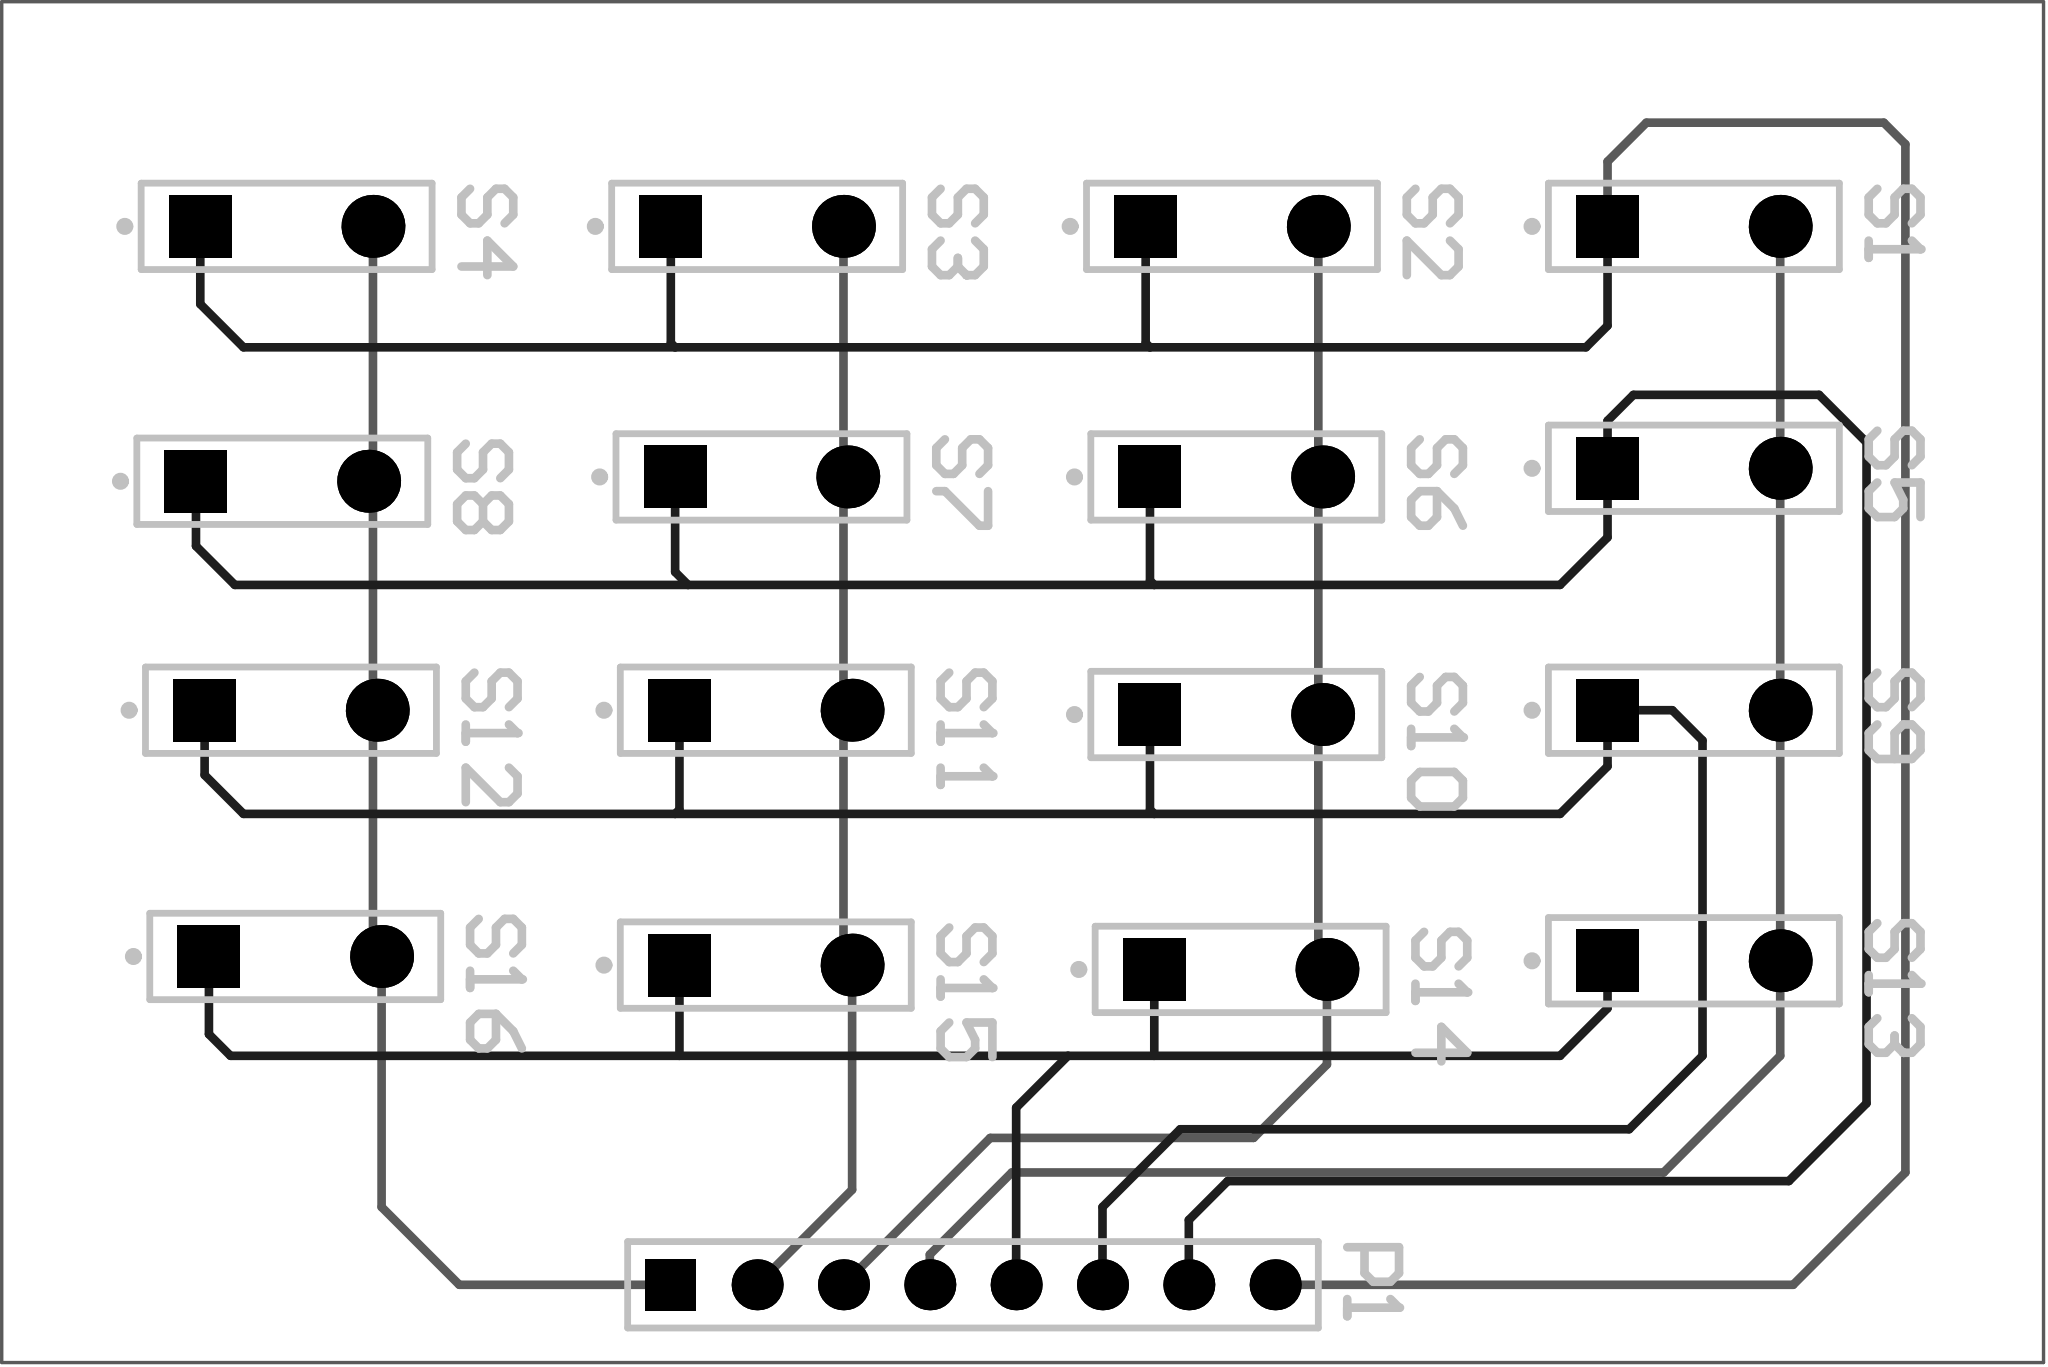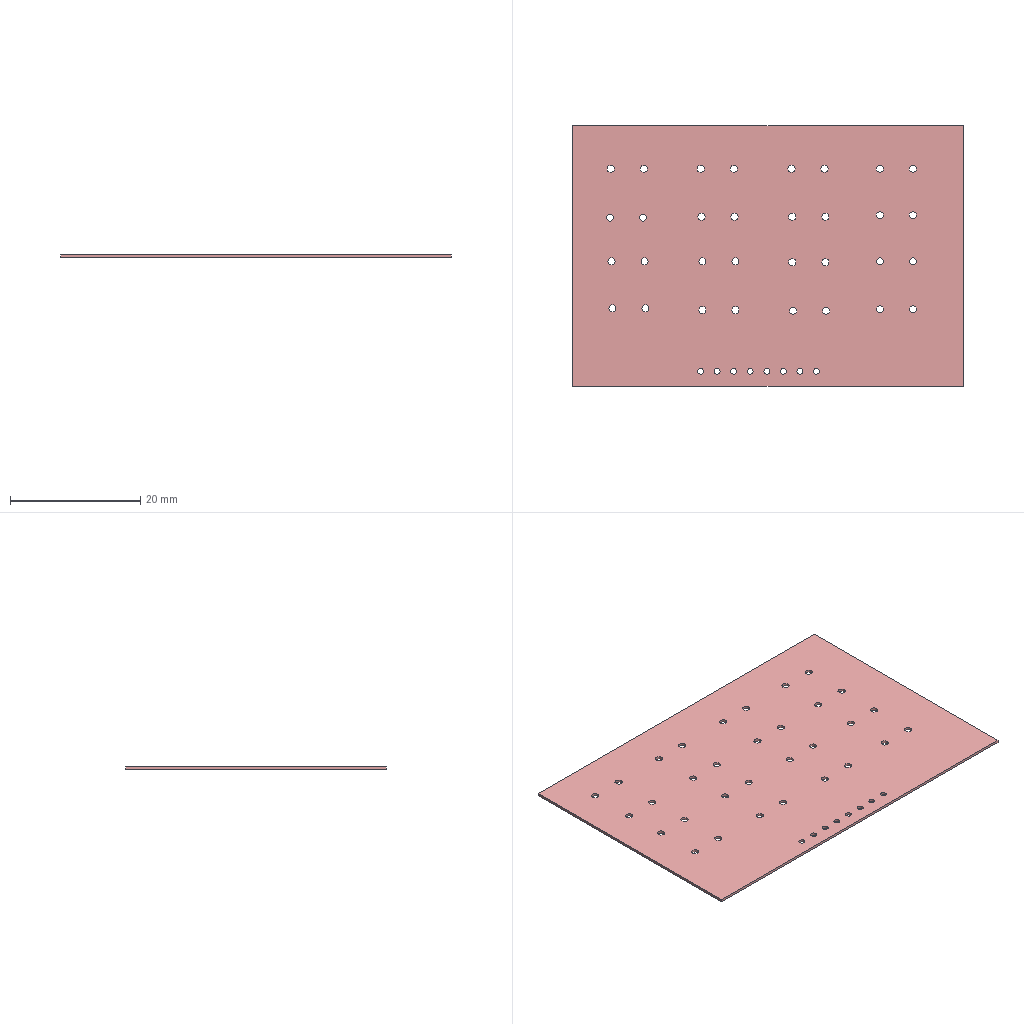Circuit board layout | Altium Designer | box 60.1 x 40 x 0.4 mm
Layer stack:
# Altium Designer layer stack of  (unit mm; dielectric type: 0 none, 1 core, 2 prepreg, 3 surface material)
index,name,kind,layer,copper_thickness_mm,dielectric_type,dielectric_thickness_mm,dielectric_material,dielectric_constant
0,Top Paste,other,,,,,,
1,Top Overlay,other,,,,,,
2,Top Solder,dielectric,,,3,0.0102,Solder Resist,3.5
3,Top Layer,copper,Top Layer,0.0356,,,,
4,Dielectric 1,dielectric,,,0,0.32,FR-4,4.8
5,Bottom Layer,copper,Bottom Layer,0.0356,,,,
6,Bottom Solder,dielectric,,,3,0.0102,Solder Resist,3.5
7,Bottom Overlay,other,,,,,,
8,Bottom Paste,other,,,,,,
# drill layer pairs: low layer,high layer
drill_pair,Top Layer,Bottom Layer
Part placement:
Designator,Comment,Layer,Footprint,Center-X(mm),Center-Y(mm),Rotation
S16,SW-PB,TopLayer,SPST-2,34.036,37.338,360
S15,SW-PB,TopLayer,SPST-2,47.879,37.084,360
S14,SW-PB,TopLayer,SPST-2,61.849,36.957,360
S13,SW-PB,TopLayer,SPST-2,75.184,37.211,360
S12,SW-PB,TopLayer,SPST-2,33.909,44.577,360
S11,SW-PB,TopLayer,SPST-2,47.879,44.577,360
S10,SW-PB,TopLayer,SPST-2,61.722,44.45,360
S9,SW-PB,TopLayer,SPST-2,75.184,44.577,360
S8,SW-PB,TopLayer,SPST-2,33.655,51.308,360
S7,SW-PB,TopLayer,SPST-2,47.752,51.435,360
S6,SW-PB,TopLayer,SPST-2,61.722,51.435,360
S5,SW-PB,TopLayer,SPST-2,75.184,51.689,360
S4,SW-PB,TopLayer,SPST-2,33.782,58.801,360
S3,SW-PB,TopLayer,SPST-2,47.625,58.801,360
S2,SW-PB,TopLayer,SPST-2,61.595,58.801,360
S1,SW-PB,TopLayer,SPST-2,75.184,58.801,360
P1,Header 8,TopLayer,HDR1X8,53.975,27.686,360
Pad and via stacks:
# Altium Designer via and pad stacks of  (unit mm). Each distinct definition once, with the count of objects using it.
# via: kind,start_layer,end_layer,hole_mm,diameter_mm,mode(0 simple;1 top-mid-bottom;2 full stack),diameter_per_layer,count,example_net
# pad: kind,layer,hole_mm,hole_type(0 round;1 square;2 slot),plating,top_size,top_shape(1 round;2 rect;3 octagon;9 rounded rect),mid_size,bottom_size,mode,footprint,size_per_layer,count,example
pad,Multi-Layer,1.1,0,plated,1.85x1.85,2,1.85x1.85,1.85x1.85,0,SPST-2,,16,S4.1
pad,Multi-Layer,1.1,0,plated,1.85x1.85,1,1.85x1.85,1.85x1.85,0,SPST-2,,16,S4.2
pad,Multi-Layer,0.9,0,plated,1.5x1.5,2,1.5x1.5,1.5x1.5,0,HDR1X8,,1,P1.1
pad,Multi-Layer,0.9,0,plated,1.5x1.5,1,1.5x1.5,1.5x1.5,0,HDR1X8,,7,P1.2
Design rules, without the lines most boards share:
# Altium Designer design rules of  (exported by Altium Designer, unit mm)
# columns: name | kind | enabled | priority | scope1 | scope2 | descriptor | typed fields (field=value)
NetAntennae | 56 | enabled | 1 | All | All | Net Antennae (Tolerance=0mm) (All) |
SilkToSilkClearance | 55 | enabled | 1 | All | All | Silk to Silk (Clearance=0mm) (All),(All) |
SilkToSolderMaskClearance | 54 | enabled | 1 | IsPad | All | Silk To Solder Mask (Clearance=0mm) (IsPad),(All) |
MinimumSolderMaskSliver | 53 | enabled | 1 | All | All | Minimum Solder Mask Sliver (Gap=0mm) (All),(All) |
HoleToHoleClearance | 52 | enabled | 1 | All | All | Hole To Hole Clearance (Gap=0.254mm) (All),(All) | gap=0.254
DiffPairsRouting | 51 | enabled | 1 | All | All | Differential Pairs Uncoupled Length using the Gap Constraints (Min=0.254mm) (Max=0.254mm) (Prefered=0.254mm)  and Width Constraints (Min=0.381mm) (Max=0.381mm) (Prefered=0.381mm) (All) |
HoleSize | 42 | enabled | 1 | All | All | Hole Size Constraint (Min=0.025mm) (Max=2.54mm) (All) |
Height | 50 | enabled | 1 | All | All | Height Constraint (Min=0mm) (Max=25.4mm) (Prefered=12.7mm) (All) | min_height=0 max_height=25.4
ComponentClearance | 24 | enabled | 1 | All | All | Component Clearance Constraint ( Horizontal Gap = 0.254mm, Vertical Gap = 0.254mm ) (All),(All)  | gap=0.254
SolderMaskExpansion | 13 | enabled | 1 | All | All | Solder Mask Expansion (Expansion =0.102mm) (All) | expansion=0.1016
PasteMaskExpansion | 14 | enabled | 1 | All | All | Paste Mask Expansion (Expansion =0mm) (All) | expansion=0
RoutingVias | 11 | enabled | 1 | All | All | Routing Via (MinHoleWidth=0.711mm) (MaxHoleWidth=0.711mm) (PreferredHoleWidth=0.711mm) (MinWidth=1.27mm) (MaxWidth=1.27mm) (PreferedWidth=1.27mm) (All) | via_min_hole=0.7112 via_max_hole=0.7112 via_preferred_diameter=1.27 via_preferred_hole=0.7112
RoutingCorners | 10 | enabled | 1 | All | All | Routing Corners (Style=45-Degree) (Min Setback=2.54mm) (Max Setback=2.54mm) (All) |
Width | 2 | enabled | 1 | All | All | Width Constraint (Min=0.254mm) (Max=0.254mm) (Preferred=0.254mm) (All) |
PolygonConnect | 20 | enabled | 1 | All | All | Polygon Connect Rule(Relief Connect )(Conductor Width=0.254mm) (Relief Angle=90 Angle) (Entries=4) (Air Gap Width=0.254mm) (All),(All) | connect_style(0=relief,1=direct,2=none)=0 relief_conductor_width=0.254 relief_entries=4
PlaneClearance | 12 | enabled | 1 | All | All | Power Plane Clearance (Clearance =0.508mm) (All) | clearance=0.508
PlaneConnect | 6 | enabled | 1 | All | All | Power Plane Connect Rule(Relief Connect )(Expansion=0.508mm) (Conductor Width=0.254mm) (Air Gap=0.254mm) (Entries=4) (All) | relief_conductor_width=0.254 relief_entries=4 relief_expansion=0.508
Clearance | 0 | enabled | 1 | All | All | Clearance Constraint (Gap=0.254mm) (All),(All) | gap=0.254
Classes set for this board:
# Altium Designer classes of  (member kind: 0 net, 1 component, 2 from-to, 3 pad, 4 layer, 5 differential pair, 6 design channel, 7 polygon, 8 structure, 9 xSignal)
# columns: class name | member kind | superclass | members
Sheet1 | 1 | no | P1; S1; S2; S3; S4; S5; S6; S7; S8; S9; S10; S11; S12; S13; S14; S15; S16;